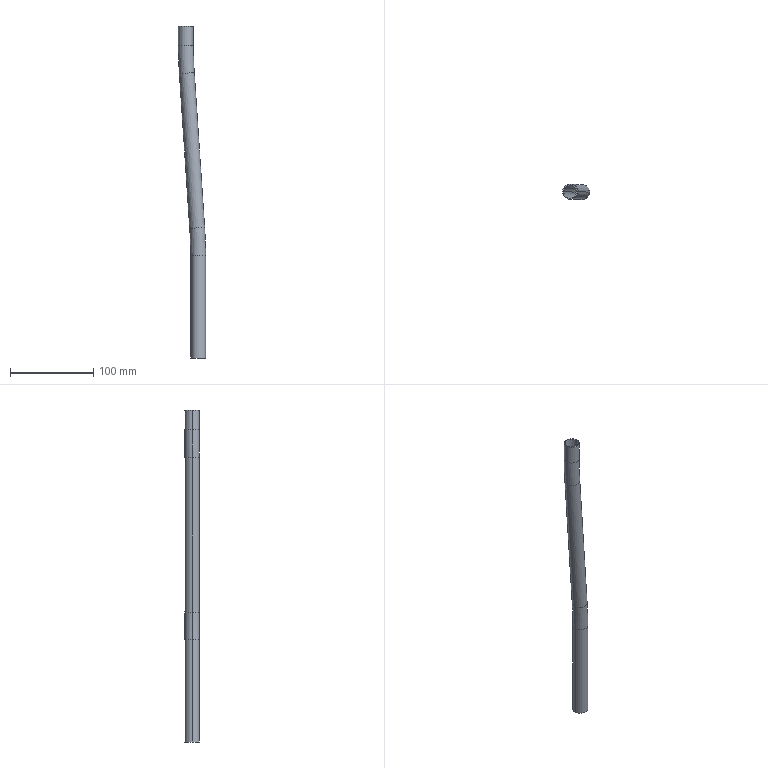Part | STEP file | Upper Chain Tube | 1 solid | 22 faces | box 32.75 x 18 x 400 mm | volume 21388 mm3 | cylinder 12 | torus 8 | plane 2 | commonest cylinder face diameters 16 x6 18 x6
STEP:
#1=CARTESIAN_POINT('',(0.,0.,0.));
#2=DIRECTION('',(0.,0.,1.));
#3=DIRECTION('',(1.,0.,0.));
#4=AXIS2_PLACEMENT_3D('',#1,#2,#3);
#5=CARTESIAN_POINT('',(-8.,0.,23.257));
#6=VERTEX_POINT('',#5);
#7=CARTESIAN_POINT('',(-9.102,0.,56.17));
#8=VERTEX_POINT('',#7);
#9=CARTESIAN_POINT('',(-500.,0.,23.257));
#10=DIRECTION('',(0.,-1.,0.));
#11=DIRECTION('',(0.,0.,-1.));
#12=AXIS2_PLACEMENT_3D('',#9,#10,#11);
#13=CIRCLE('',#12,492.);
#14=CARTESIAN_POINT('',(-500.,0.,23.257));
#15=DIRECTION('',(0.,-1.,0.));
#16=DIRECTION('',(0.,0.,-1.));
#17=AXIS2_PLACEMENT_3D('',#14,#15,#16);
#18=TOROIDAL_SURFACE('',#17,500.,8.);
#19=CARTESIAN_POINT('',(0.,3.142));
#20=DIRECTION('',(1.,0.));
#21=VECTOR('',#20,1.);
#22=LINE('',#19,#21);
#23=(GEOMETRIC_REPRESENTATION_CONTEXT(2)PARAMETRIC_REPRESENTATION_CONTEXT()REPRESENTATION_CONTEXT('',''));
#24=DEFINITIONAL_REPRESENTATION('',(#22),#23);
#25=PCURVE('',#18,#24);
#26=CARTESIAN_POINT('',(-500.,0.,23.257));
#27=DIRECTION('',(0.,-1.,0.));
#28=DIRECTION('',(0.,0.,-1.));
#29=AXIS2_PLACEMENT_3D('',#26,#27,#28);
#30=TOROIDAL_SURFACE('',#29,500.,8.);
#31=CARTESIAN_POINT('',(0.,3.142));
#32=DIRECTION('',(1.,0.));
#33=VECTOR('',#32,1.);
#34=LINE('',#31,#33);
#35=(GEOMETRIC_REPRESENTATION_CONTEXT(2)PARAMETRIC_REPRESENTATION_CONTEXT()REPRESENTATION_CONTEXT('',''));
#36=DEFINITIONAL_REPRESENTATION('',(#34),#35);
#37=PCURVE('',#30,#36);
#38=SURFACE_CURVE('',#13,(#25,#37),.PCURVE_S1.);
#39=EDGE_CURVE('',#6,#8,#38,.T.);
#40=ORIENTED_EDGE('',*,*,#39,.T.);
#41=CARTESIAN_POINT('',(6.862,0.,57.24));
#42=VERTEX_POINT('',#41);
#43=CARTESIAN_POINT('',(-1.12,0.,56.705));
#44=DIRECTION('',(-0.0669,0.,0.9978));
#45=DIRECTION('',(0.9978,0.,0.0669));
#46=AXIS2_PLACEMENT_3D('',#43,#44,#45);
#47=CIRCLE('',#46,8.);
#48=CARTESIAN_POINT('',(1.638,6.283));
#49=DIRECTION('',(0.,-1.));
#50=VECTOR('',#49,1.);
#51=LINE('',#48,#50);
#52=(GEOMETRIC_REPRESENTATION_CONTEXT(2)PARAMETRIC_REPRESENTATION_CONTEXT()REPRESENTATION_CONTEXT('',''));
#53=DEFINITIONAL_REPRESENTATION('',(#51),#52);
#54=PCURVE('',#18,#53);
#55=CARTESIAN_POINT('',(-1.12,0.,56.705));
#56=DIRECTION('',(-0.0669,0.,0.9978));
#57=DIRECTION('',(0.9978,0.,0.0669));
#58=AXIS2_PLACEMENT_3D('',#55,#56,#57);
#59=CYLINDRICAL_SURFACE('',#58,8.);
#60=CARTESIAN_POINT('',(0.,0.));
#61=DIRECTION('',(1.,0.));
#62=VECTOR('',#61,1.);
#63=LINE('',#60,#62);
#64=(GEOMETRIC_REPRESENTATION_CONTEXT(2)PARAMETRIC_REPRESENTATION_CONTEXT()REPRESENTATION_CONTEXT('',''));
#65=DEFINITIONAL_REPRESENTATION('',(#63),#64);
#66=PCURVE('',#59,#65);
#67=SURFACE_CURVE('',#47,(#54,#66),.PCURVE_S1.);
#68=EDGE_CURVE('',#42,#8,#67,.T.);
#69=ORIENTED_EDGE('',*,*,#68,.F.);
#70=CARTESIAN_POINT('',(8.,0.,23.257));
#71=VERTEX_POINT('',#70);
#72=CARTESIAN_POINT('',(-500.,0.,23.257));
#73=DIRECTION('',(0.,-1.,0.));
#74=DIRECTION('',(0.,0.,-1.));
#75=AXIS2_PLACEMENT_3D('',#72,#73,#74);
#76=CIRCLE('',#75,508.);
#77=CARTESIAN_POINT('',(0.,6.283));
#78=DIRECTION('',(1.,0.));
#79=VECTOR('',#78,1.);
#80=LINE('',#77,#79);
#81=(GEOMETRIC_REPRESENTATION_CONTEXT(2)PARAMETRIC_REPRESENTATION_CONTEXT()REPRESENTATION_CONTEXT('',''));
#82=DEFINITIONAL_REPRESENTATION('',(#80),#81);
#83=PCURVE('',#18,#82);
#84=CARTESIAN_POINT('',(0.,0.));
#85=DIRECTION('',(1.,0.));
#86=VECTOR('',#85,1.);
#87=LINE('',#84,#86);
#88=(GEOMETRIC_REPRESENTATION_CONTEXT(2)PARAMETRIC_REPRESENTATION_CONTEXT()REPRESENTATION_CONTEXT('',''));
#89=DEFINITIONAL_REPRESENTATION('',(#87),#88);
#90=PCURVE('',#30,#89);
#91=SURFACE_CURVE('',#76,(#83,#90),.PCURVE_S1.);
#92=EDGE_CURVE('',#71,#42,#91,.T.);
#93=ORIENTED_EDGE('',*,*,#92,.F.);
#94=CARTESIAN_POINT('',(0.,0.,23.257));
#95=DIRECTION('',(0.,0.,1.));
#96=DIRECTION('',(1.,0.,0.));
#97=AXIS2_PLACEMENT_3D('',#94,#95,#96);
#98=CIRCLE('',#97,8.);
#99=CARTESIAN_POINT('',(1.571,6.283));
#100=DIRECTION('',(0.,-1.));
#101=VECTOR('',#100,1.);
#102=LINE('',#99,#101);
#103=(GEOMETRIC_REPRESENTATION_CONTEXT(2)PARAMETRIC_REPRESENTATION_CONTEXT()REPRESENTATION_CONTEXT('',''));
#104=DEFINITIONAL_REPRESENTATION('',(#102),#103);
#105=PCURVE('',#18,#104);
#106=CARTESIAN_POINT('',(0.,0.,-100.));
#107=DIRECTION('',(0.,0.,1.));
#108=DIRECTION('',(1.,0.,0.));
#109=AXIS2_PLACEMENT_3D('',#106,#107,#108);
#110=CYLINDRICAL_SURFACE('',#109,8.);
#111=CARTESIAN_POINT('',(0.,123.257));
#112=DIRECTION('',(1.,0.));
#113=VECTOR('',#112,1.);
#114=LINE('',#111,#113);
#115=(GEOMETRIC_REPRESENTATION_CONTEXT(2)PARAMETRIC_REPRESENTATION_CONTEXT()REPRESENTATION_CONTEXT('',''));
#116=DEFINITIONAL_REPRESENTATION('',(#114),#115);
#117=PCURVE('',#110,#116);
#118=SURFACE_CURVE('',#98,(#105,#117),.PCURVE_S1.);
#119=EDGE_CURVE('',#71,#6,#118,.T.);
#120=ORIENTED_EDGE('',*,*,#119,.T.);
#121=EDGE_LOOP('',(#40,#69,#93,#120));
#122=FACE_BOUND('',#121,.F.);
#123=ADVANCED_FACE('',(#122),#18,.F.);
#124=CARTESIAN_POINT('',(-9.,0.,23.257));
#125=VERTEX_POINT('',#124);
#126=CARTESIAN_POINT('',(9.,0.,23.257));
#127=VERTEX_POINT('',#126);
#128=CARTESIAN_POINT('',(0.,0.,23.257));
#129=DIRECTION('',(0.,0.,1.));
#130=DIRECTION('',(1.,0.,0.));
#131=AXIS2_PLACEMENT_3D('',#128,#129,#130);
#132=CIRCLE('',#131,9.);
#133=CARTESIAN_POINT('',(-500.,0.,23.257));
#134=DIRECTION('',(0.,-1.,0.));
#135=DIRECTION('',(0.,0.,-1.));
#136=AXIS2_PLACEMENT_3D('',#133,#134,#135);
#137=TOROIDAL_SURFACE('',#136,500.,9.);
#138=CARTESIAN_POINT('',(1.571,6.283));
#139=DIRECTION('',(0.,-1.));
#140=VECTOR('',#139,1.);
#141=LINE('',#138,#140);
#142=(GEOMETRIC_REPRESENTATION_CONTEXT(2)PARAMETRIC_REPRESENTATION_CONTEXT()REPRESENTATION_CONTEXT('',''));
#143=DEFINITIONAL_REPRESENTATION('',(#141),#142);
#144=PCURVE('',#137,#143);
#145=CARTESIAN_POINT('',(0.,0.,-100.));
#146=DIRECTION('',(0.,0.,1.));
#147=DIRECTION('',(1.,0.,0.));
#148=AXIS2_PLACEMENT_3D('',#145,#146,#147);
#149=CYLINDRICAL_SURFACE('',#148,9.);
#150=CARTESIAN_POINT('',(0.,123.257));
#151=DIRECTION('',(1.,0.));
#152=VECTOR('',#151,1.);
#153=LINE('',#150,#152);
#154=(GEOMETRIC_REPRESENTATION_CONTEXT(2)PARAMETRIC_REPRESENTATION_CONTEXT()REPRESENTATION_CONTEXT('',''));
#155=DEFINITIONAL_REPRESENTATION('',(#153),#154);
#156=PCURVE('',#149,#155);
#157=SURFACE_CURVE('',#132,(#144,#156),.PCURVE_S1.);
#158=EDGE_CURVE('',#125,#127,#157,.T.);
#159=ORIENTED_EDGE('',*,*,#158,.T.);
#160=CARTESIAN_POINT('',(7.86,0.,57.307));
#161=VERTEX_POINT('',#160);
#162=CARTESIAN_POINT('',(-500.,0.,23.257));
#163=DIRECTION('',(0.,-1.,0.));
#164=DIRECTION('',(0.,0.,-1.));
#165=AXIS2_PLACEMENT_3D('',#162,#163,#164);
#166=CIRCLE('',#165,509.);
#167=CARTESIAN_POINT('',(0.,0.));
#168=DIRECTION('',(1.,0.));
#169=VECTOR('',#168,1.);
#170=LINE('',#167,#169);
#171=(GEOMETRIC_REPRESENTATION_CONTEXT(2)PARAMETRIC_REPRESENTATION_CONTEXT()REPRESENTATION_CONTEXT('',''));
#172=DEFINITIONAL_REPRESENTATION('',(#170),#171);
#173=PCURVE('',#137,#172);
#174=CARTESIAN_POINT('',(-500.,0.,23.257));
#175=DIRECTION('',(0.,-1.,0.));
#176=DIRECTION('',(0.,0.,-1.));
#177=AXIS2_PLACEMENT_3D('',#174,#175,#176);
#178=TOROIDAL_SURFACE('',#177,500.,9.);
#179=CARTESIAN_POINT('',(0.,6.283));
#180=DIRECTION('',(1.,0.));
#181=VECTOR('',#180,1.);
#182=LINE('',#179,#181);
#183=(GEOMETRIC_REPRESENTATION_CONTEXT(2)PARAMETRIC_REPRESENTATION_CONTEXT()REPRESENTATION_CONTEXT('',''));
#184=DEFINITIONAL_REPRESENTATION('',(#182),#183);
#185=PCURVE('',#178,#184);
#186=SURFACE_CURVE('',#166,(#173,#185),.PCURVE_S1.);
#187=EDGE_CURVE('',#127,#161,#186,.T.);
#188=ORIENTED_EDGE('',*,*,#187,.T.);
#189=CARTESIAN_POINT('',(-10.1,0.,56.103));
#190=VERTEX_POINT('',#189);
#191=CARTESIAN_POINT('',(-1.12,0.,56.705));
#192=DIRECTION('',(-0.0669,0.,0.9978));
#193=DIRECTION('',(0.9978,0.,0.0669));
#194=AXIS2_PLACEMENT_3D('',#191,#192,#193);
#195=CIRCLE('',#194,9.);
#196=CARTESIAN_POINT('',(1.638,6.283));
#197=DIRECTION('',(0.,-1.));
#198=VECTOR('',#197,1.);
#199=LINE('',#196,#198);
#200=(GEOMETRIC_REPRESENTATION_CONTEXT(2)PARAMETRIC_REPRESENTATION_CONTEXT()REPRESENTATION_CONTEXT('',''));
#201=DEFINITIONAL_REPRESENTATION('',(#199),#200);
#202=PCURVE('',#137,#201);
#203=CARTESIAN_POINT('',(-1.12,0.,56.705));
#204=DIRECTION('',(-0.0669,0.,0.9978));
#205=DIRECTION('',(0.9978,0.,0.0669));
#206=AXIS2_PLACEMENT_3D('',#203,#204,#205);
#207=CYLINDRICAL_SURFACE('',#206,9.);
#208=CARTESIAN_POINT('',(0.,0.));
#209=DIRECTION('',(1.,0.));
#210=VECTOR('',#209,1.);
#211=LINE('',#208,#210);
#212=(GEOMETRIC_REPRESENTATION_CONTEXT(2)PARAMETRIC_REPRESENTATION_CONTEXT()REPRESENTATION_CONTEXT('',''));
#213=DEFINITIONAL_REPRESENTATION('',(#211),#212);
#214=PCURVE('',#207,#213);
#215=SURFACE_CURVE('',#195,(#202,#214),.PCURVE_S1.);
#216=EDGE_CURVE('',#190,#161,#215,.T.);
#217=ORIENTED_EDGE('',*,*,#216,.F.);
#218=CARTESIAN_POINT('',(-500.,0.,23.257));
#219=DIRECTION('',(0.,-1.,0.));
#220=DIRECTION('',(0.,0.,-1.));
#221=AXIS2_PLACEMENT_3D('',#218,#219,#220);
#222=CIRCLE('',#221,491.);
#223=CARTESIAN_POINT('',(0.,3.142));
#224=DIRECTION('',(1.,0.));
#225=VECTOR('',#224,1.);
#226=LINE('',#223,#225);
#227=(GEOMETRIC_REPRESENTATION_CONTEXT(2)PARAMETRIC_REPRESENTATION_CONTEXT()REPRESENTATION_CONTEXT('',''));
#228=DEFINITIONAL_REPRESENTATION('',(#226),#227);
#229=PCURVE('',#137,#228);
#230=CARTESIAN_POINT('',(0.,3.142));
#231=DIRECTION('',(1.,0.));
#232=VECTOR('',#231,1.);
#233=LINE('',#230,#232);
#234=(GEOMETRIC_REPRESENTATION_CONTEXT(2)PARAMETRIC_REPRESENTATION_CONTEXT()REPRESENTATION_CONTEXT('',''));
#235=DEFINITIONAL_REPRESENTATION('',(#233),#234);
#236=PCURVE('',#178,#235);
#237=SURFACE_CURVE('',#222,(#229,#236),.PCURVE_S1.);
#238=EDGE_CURVE('',#125,#190,#237,.T.);
#239=ORIENTED_EDGE('',*,*,#238,.F.);
#240=EDGE_LOOP('',(#159,#188,#217,#239));
#241=FACE_BOUND('',#240,.T.);
#242=ADVANCED_FACE('',(#241),#137,.T.);
#243=CARTESIAN_POINT('',(-5.648,0.,243.83));
#244=VERTEX_POINT('',#243);
#245=CARTESIAN_POINT('',(-6.75,0.,276.743));
#246=VERTEX_POINT('',#245);
#247=CARTESIAN_POINT('',(485.25,0.,276.743));
#248=DIRECTION('',(0.,1.,0.));
#249=DIRECTION('',(0.,0.,1.));
#250=AXIS2_PLACEMENT_3D('',#247,#248,#249);
#251=CIRCLE('',#250,492.);
#252=CARTESIAN_POINT('',(485.25,0.,276.743));
#253=DIRECTION('',(0.,1.,0.));
#254=DIRECTION('',(0.,0.,1.));
#255=AXIS2_PLACEMENT_3D('',#252,#253,#254);
#256=TOROIDAL_SURFACE('',#255,500.,8.);
#257=CARTESIAN_POINT('',(0.,3.142));
#258=DIRECTION('',(1.,0.));
#259=VECTOR('',#258,1.);
#260=LINE('',#257,#259);
#261=(GEOMETRIC_REPRESENTATION_CONTEXT(2)PARAMETRIC_REPRESENTATION_CONTEXT()REPRESENTATION_CONTEXT('',''));
#262=DEFINITIONAL_REPRESENTATION('',(#260),#261);
#263=PCURVE('',#256,#262);
#264=CARTESIAN_POINT('',(485.25,0.,276.743));
#265=DIRECTION('',(0.,1.,0.));
#266=DIRECTION('',(0.,0.,1.));
#267=AXIS2_PLACEMENT_3D('',#264,#265,#266);
#268=TOROIDAL_SURFACE('',#267,500.,8.);
#269=CARTESIAN_POINT('',(0.,3.142));
#270=DIRECTION('',(1.,0.));
#271=VECTOR('',#270,1.);
#272=LINE('',#269,#271);
#273=(GEOMETRIC_REPRESENTATION_CONTEXT(2)PARAMETRIC_REPRESENTATION_CONTEXT()REPRESENTATION_CONTEXT('',''));
#274=DEFINITIONAL_REPRESENTATION('',(#272),#273);
#275=PCURVE('',#268,#274);
#276=SURFACE_CURVE('',#251,(#263,#275),.PCURVE_S1.);
#277=EDGE_CURVE('',#244,#246,#276,.T.);
#278=ORIENTED_EDGE('',*,*,#277,.T.);
#279=CARTESIAN_POINT('',(-22.75,0.,276.743));
#280=VERTEX_POINT('',#279);
#281=CARTESIAN_POINT('',(-14.75,0.,276.743));
#282=DIRECTION('',(0.,0.,1.));
#283=DIRECTION('',(1.,0.,0.));
#284=AXIS2_PLACEMENT_3D('',#281,#282,#283);
#285=CIRCLE('',#284,8.);
#286=CARTESIAN_POINT('',(4.712,9.425));
#287=DIRECTION('',(0.,-1.));
#288=VECTOR('',#287,1.);
#289=LINE('',#286,#288);
#290=(GEOMETRIC_REPRESENTATION_CONTEXT(2)PARAMETRIC_REPRESENTATION_CONTEXT()REPRESENTATION_CONTEXT('',''));
#291=DEFINITIONAL_REPRESENTATION('',(#289),#290);
#292=PCURVE('',#256,#291);
#293=CARTESIAN_POINT('',(-14.75,0.,276.743));
#294=DIRECTION('',(0.,0.,1.));
#295=DIRECTION('',(1.,0.,0.));
#296=AXIS2_PLACEMENT_3D('',#293,#294,#295);
#297=CYLINDRICAL_SURFACE('',#296,8.);
#298=CARTESIAN_POINT('',(0.,0.));
#299=DIRECTION('',(1.,0.));
#300=VECTOR('',#299,1.);
#301=LINE('',#298,#300);
#302=(GEOMETRIC_REPRESENTATION_CONTEXT(2)PARAMETRIC_REPRESENTATION_CONTEXT()REPRESENTATION_CONTEXT('',''));
#303=DEFINITIONAL_REPRESENTATION('',(#301),#302);
#304=PCURVE('',#297,#303);
#305=SURFACE_CURVE('',#285,(#292,#304),.PCURVE_S1.);
#306=EDGE_CURVE('',#280,#246,#305,.T.);
#307=ORIENTED_EDGE('',*,*,#306,.F.);
#308=CARTESIAN_POINT('',(-21.612,0.,242.76));
#309=VERTEX_POINT('',#308);
#310=CARTESIAN_POINT('',(485.25,0.,276.743));
#311=DIRECTION('',(0.,1.,0.));
#312=DIRECTION('',(0.,0.,1.));
#313=AXIS2_PLACEMENT_3D('',#310,#311,#312);
#314=CIRCLE('',#313,508.);
#315=CARTESIAN_POINT('',(0.,6.283));
#316=DIRECTION('',(1.,0.));
#317=VECTOR('',#316,1.);
#318=LINE('',#315,#317);
#319=(GEOMETRIC_REPRESENTATION_CONTEXT(2)PARAMETRIC_REPRESENTATION_CONTEXT()REPRESENTATION_CONTEXT('',''));
#320=DEFINITIONAL_REPRESENTATION('',(#318),#319);
#321=PCURVE('',#256,#320);
#322=CARTESIAN_POINT('',(0.,0.));
#323=DIRECTION('',(1.,0.));
#324=VECTOR('',#323,1.);
#325=LINE('',#322,#324);
#326=(GEOMETRIC_REPRESENTATION_CONTEXT(2)PARAMETRIC_REPRESENTATION_CONTEXT()REPRESENTATION_CONTEXT('',''));
#327=DEFINITIONAL_REPRESENTATION('',(#325),#326);
#328=PCURVE('',#268,#327);
#329=SURFACE_CURVE('',#314,(#321,#328),.PCURVE_S1.);
#330=EDGE_CURVE('',#309,#280,#329,.T.);
#331=ORIENTED_EDGE('',*,*,#330,.F.);
#332=CARTESIAN_POINT('',(-13.63,0.,243.295));
#333=DIRECTION('',(-0.0669,0.,0.9978));
#334=DIRECTION('',(0.9978,0.,0.0669));
#335=AXIS2_PLACEMENT_3D('',#332,#333,#334);
#336=CIRCLE('',#335,8.);
#337=CARTESIAN_POINT('',(4.645,9.425));
#338=DIRECTION('',(0.,-1.));
#339=VECTOR('',#338,1.);
#340=LINE('',#337,#339);
#341=(GEOMETRIC_REPRESENTATION_CONTEXT(2)PARAMETRIC_REPRESENTATION_CONTEXT()REPRESENTATION_CONTEXT('',''));
#342=DEFINITIONAL_REPRESENTATION('',(#340),#341);
#343=PCURVE('',#256,#342);
#344=CARTESIAN_POINT('',(-1.12,0.,56.705));
#345=DIRECTION('',(-0.0669,0.,0.9978));
#346=DIRECTION('',(0.9978,0.,0.0669));
#347=AXIS2_PLACEMENT_3D('',#344,#345,#346);
#348=CYLINDRICAL_SURFACE('',#347,8.);
#349=CARTESIAN_POINT('',(0.,187.009));
#350=DIRECTION('',(1.,0.));
#351=VECTOR('',#350,1.);
#352=LINE('',#349,#351);
#353=(GEOMETRIC_REPRESENTATION_CONTEXT(2)PARAMETRIC_REPRESENTATION_CONTEXT()REPRESENTATION_CONTEXT('',''));
#354=DEFINITIONAL_REPRESENTATION('',(#352),#353);
#355=PCURVE('',#348,#354);
#356=SURFACE_CURVE('',#336,(#343,#355),.PCURVE_S1.);
#357=EDGE_CURVE('',#309,#244,#356,.T.);
#358=ORIENTED_EDGE('',*,*,#357,.T.);
#359=EDGE_LOOP('',(#278,#307,#331,#358));
#360=FACE_BOUND('',#359,.F.);
#361=ADVANCED_FACE('',(#360),#256,.F.);
#362=CARTESIAN_POINT('',(-4.65,0.,243.897));
#363=VERTEX_POINT('',#362);
#364=CARTESIAN_POINT('',(-22.61,0.,242.693));
#365=VERTEX_POINT('',#364);
#366=CARTESIAN_POINT('',(-13.63,0.,243.295));
#367=DIRECTION('',(-0.0669,0.,0.9978));
#368=DIRECTION('',(0.9978,0.,0.0669));
#369=AXIS2_PLACEMENT_3D('',#366,#367,#368);
#370=CIRCLE('',#369,9.);
#371=CARTESIAN_POINT('',(485.25,0.,276.743));
#372=DIRECTION('',(0.,1.,0.));
#373=DIRECTION('',(0.,0.,1.));
#374=AXIS2_PLACEMENT_3D('',#371,#372,#373);
#375=TOROIDAL_SURFACE('',#374,500.,9.);
#376=CARTESIAN_POINT('',(4.645,3.142));
#377=DIRECTION('',(0.,-1.));
#378=VECTOR('',#377,1.);
#379=LINE('',#376,#378);
#380=(GEOMETRIC_REPRESENTATION_CONTEXT(2)PARAMETRIC_REPRESENTATION_CONTEXT()REPRESENTATION_CONTEXT('',''));
#381=DEFINITIONAL_REPRESENTATION('',(#379),#380);
#382=PCURVE('',#375,#381);
#383=CARTESIAN_POINT('',(-1.12,0.,56.705));
#384=DIRECTION('',(-0.0669,0.,0.9978));
#385=DIRECTION('',(0.9978,0.,0.0669));
#386=AXIS2_PLACEMENT_3D('',#383,#384,#385);
#387=CYLINDRICAL_SURFACE('',#386,9.);
#388=CARTESIAN_POINT('',(0.,187.009));
#389=DIRECTION('',(1.,0.));
#390=VECTOR('',#389,1.);
#391=LINE('',#388,#390);
#392=(GEOMETRIC_REPRESENTATION_CONTEXT(2)PARAMETRIC_REPRESENTATION_CONTEXT()REPRESENTATION_CONTEXT('',''));
#393=DEFINITIONAL_REPRESENTATION('',(#391),#392);
#394=PCURVE('',#387,#393);
#395=SURFACE_CURVE('',#370,(#382,#394),.PCURVE_S1.);
#396=EDGE_CURVE('',#363,#365,#395,.T.);
#397=ORIENTED_EDGE('',*,*,#396,.T.);
#398=CARTESIAN_POINT('',(-23.75,0.,276.743));
#399=VERTEX_POINT('',#398);
#400=CARTESIAN_POINT('',(485.25,0.,276.743));
#401=DIRECTION('',(0.,1.,0.));
#402=DIRECTION('',(0.,0.,1.));
#403=AXIS2_PLACEMENT_3D('',#400,#401,#402);
#404=CIRCLE('',#403,509.);
#405=CARTESIAN_POINT('',(0.,0.));
#406=DIRECTION('',(1.,0.));
#407=VECTOR('',#406,1.);
#408=LINE('',#405,#407);
#409=(GEOMETRIC_REPRESENTATION_CONTEXT(2)PARAMETRIC_REPRESENTATION_CONTEXT()REPRESENTATION_CONTEXT('',''));
#410=DEFINITIONAL_REPRESENTATION('',(#408),#409);
#411=PCURVE('',#375,#410);
#412=CARTESIAN_POINT('',(485.25,0.,276.743));
#413=DIRECTION('',(0.,1.,0.));
#414=DIRECTION('',(0.,0.,1.));
#415=AXIS2_PLACEMENT_3D('',#412,#413,#414);
#416=TOROIDAL_SURFACE('',#415,500.,9.);
#417=CARTESIAN_POINT('',(0.,6.283));
#418=DIRECTION('',(1.,0.));
#419=VECTOR('',#418,1.);
#420=LINE('',#417,#419);
#421=(GEOMETRIC_REPRESENTATION_CONTEXT(2)PARAMETRIC_REPRESENTATION_CONTEXT()REPRESENTATION_CONTEXT('',''));
#422=DEFINITIONAL_REPRESENTATION('',(#420),#421);
#423=PCURVE('',#416,#422);
#424=SURFACE_CURVE('',#404,(#411,#423),.PCURVE_S1.);
#425=EDGE_CURVE('',#365,#399,#424,.T.);
#426=ORIENTED_EDGE('',*,*,#425,.T.);
#427=CARTESIAN_POINT('',(-5.75,0.,276.743));
#428=VERTEX_POINT('',#427);
#429=CARTESIAN_POINT('',(-14.75,0.,276.743));
#430=DIRECTION('',(0.,0.,1.));
#431=DIRECTION('',(1.,0.,0.));
#432=AXIS2_PLACEMENT_3D('',#429,#430,#431);
#433=CIRCLE('',#432,9.);
#434=CARTESIAN_POINT('',(4.712,3.142));
#435=DIRECTION('',(0.,-1.));
#436=VECTOR('',#435,1.);
#437=LINE('',#434,#436);
#438=(GEOMETRIC_REPRESENTATION_CONTEXT(2)PARAMETRIC_REPRESENTATION_CONTEXT()REPRESENTATION_CONTEXT('',''));
#439=DEFINITIONAL_REPRESENTATION('',(#437),#438);
#440=PCURVE('',#375,#439);
#441=CARTESIAN_POINT('',(-14.75,0.,276.743));
#442=DIRECTION('',(0.,0.,1.));
#443=DIRECTION('',(1.,0.,0.));
#444=AXIS2_PLACEMENT_3D('',#441,#442,#443);
#445=CYLINDRICAL_SURFACE('',#444,9.);
#446=CARTESIAN_POINT('',(0.,0.));
#447=DIRECTION('',(1.,0.));
#448=VECTOR('',#447,1.);
#449=LINE('',#446,#448);
#450=(GEOMETRIC_REPRESENTATION_CONTEXT(2)PARAMETRIC_REPRESENTATION_CONTEXT()REPRESENTATION_CONTEXT('',''));
#451=DEFINITIONAL_REPRESENTATION('',(#449),#450);
#452=PCURVE('',#445,#451);
#453=SURFACE_CURVE('',#433,(#440,#452),.PCURVE_S1.);
#454=EDGE_CURVE('',#428,#399,#453,.T.);
#455=ORIENTED_EDGE('',*,*,#454,.F.);
#456=CARTESIAN_POINT('',(485.25,0.,276.743));
#457=DIRECTION('',(0.,1.,0.));
#458=DIRECTION('',(0.,0.,1.));
#459=AXIS2_PLACEMENT_3D('',#456,#457,#458);
#460=CIRCLE('',#459,491.);
#461=CARTESIAN_POINT('',(0.,3.142));
#462=DIRECTION('',(1.,0.));
#463=VECTOR('',#462,1.);
#464=LINE('',#461,#463);
#465=(GEOMETRIC_REPRESENTATION_CONTEXT(2)PARAMETRIC_REPRESENTATION_CONTEXT()REPRESENTATION_CONTEXT('',''));
#466=DEFINITIONAL_REPRESENTATION('',(#464),#465);
#467=PCURVE('',#375,#466);
#468=CARTESIAN_POINT('',(0.,3.142));
#469=DIRECTION('',(1.,0.));
#470=VECTOR('',#469,1.);
#471=LINE('',#468,#470);
#472=(GEOMETRIC_REPRESENTATION_CONTEXT(2)PARAMETRIC_REPRESENTATION_CONTEXT()REPRESENTATION_CONTEXT('',''));
#473=DEFINITIONAL_REPRESENTATION('',(#471),#472);
#474=PCURVE('',#416,#473);
#475=SURFACE_CURVE('',#460,(#467,#474),.PCURVE_S1.);
#476=EDGE_CURVE('',#363,#428,#475,.T.);
#477=ORIENTED_EDGE('',*,*,#476,.F.);
#478=EDGE_LOOP('',(#397,#426,#455,#477));
#479=FACE_BOUND('',#478,.T.);
#480=ADVANCED_FACE('',(#479),#375,.T.);
#481=CARTESIAN_POINT('',(6.862,0.,57.24));
#482=DIRECTION('',(-0.0669,0.,0.9978));
#483=VECTOR('',#482,1.);
#484=LINE('',#481,#483);
#485=CARTESIAN_POINT('',(6.283,0.));
#486=DIRECTION('',(0.,1.));
#487=VECTOR('',#486,1.);
#488=LINE('',#485,#487);
#489=(GEOMETRIC_REPRESENTATION_CONTEXT(2)PARAMETRIC_REPRESENTATION_CONTEXT()REPRESENTATION_CONTEXT('',''));
#490=DEFINITIONAL_REPRESENTATION('',(#488),#489);
#491=PCURVE('',#348,#490);
#492=CARTESIAN_POINT('',(0.,0.));
#493=DIRECTION('',(0.,1.));
#494=VECTOR('',#493,1.);
#495=LINE('',#492,#494);
#496=(GEOMETRIC_REPRESENTATION_CONTEXT(2)PARAMETRIC_REPRESENTATION_CONTEXT()REPRESENTATION_CONTEXT('',''));
#497=DEFINITIONAL_REPRESENTATION('',(#495),#496);
#498=PCURVE('',#59,#497);
#499=SURFACE_CURVE('',#484,(#491,#498),.PCURVE_S1.);
#500=EDGE_CURVE('',#42,#244,#499,.T.);
#501=ORIENTED_EDGE('',*,*,#500,.T.);
#502=ORIENTED_EDGE('',*,*,#357,.F.);
#503=CARTESIAN_POINT('',(-9.102,0.,56.17));
#504=DIRECTION('',(-0.0669,0.,0.9978));
#505=VECTOR('',#504,1.);
#506=LINE('',#503,#505);
#507=CARTESIAN_POINT('',(3.142,0.));
#508=DIRECTION('',(0.,1.));
#509=VECTOR('',#508,1.);
#510=LINE('',#507,#509);
#511=(GEOMETRIC_REPRESENTATION_CONTEXT(2)PARAMETRIC_REPRESENTATION_CONTEXT()REPRESENTATION_CONTEXT('',''));
#512=DEFINITIONAL_REPRESENTATION('',(#510),#511);
#513=PCURVE('',#348,#512);
#514=CARTESIAN_POINT('',(3.142,0.));
#515=DIRECTION('',(0.,1.));
#516=VECTOR('',#515,1.);
#517=LINE('',#514,#516);
#518=(GEOMETRIC_REPRESENTATION_CONTEXT(2)PARAMETRIC_REPRESENTATION_CONTEXT()REPRESENTATION_CONTEXT('',''));
#519=DEFINITIONAL_REPRESENTATION('',(#517),#518);
#520=PCURVE('',#59,#519);
#521=SURFACE_CURVE('',#506,(#513,#520),.PCURVE_S1.);
#522=EDGE_CURVE('',#8,#309,#521,.T.);
#523=ORIENTED_EDGE('',*,*,#522,.F.);
#524=CARTESIAN_POINT('',(-1.12,0.,56.705));
#525=DIRECTION('',(-0.0669,0.,0.9978));
#526=DIRECTION('',(0.9978,0.,0.0669));
#527=AXIS2_PLACEMENT_3D('',#524,#525,#526);
#528=CIRCLE('',#527,8.);
#529=CARTESIAN_POINT('',(0.,0.));
#530=DIRECTION('',(1.,0.));
#531=VECTOR('',#530,1.);
#532=LINE('',#529,#531);
#533=(GEOMETRIC_REPRESENTATION_CONTEXT(2)PARAMETRIC_REPRESENTATION_CONTEXT()REPRESENTATION_CONTEXT('',''));
#534=DEFINITIONAL_REPRESENTATION('',(#532),#533);
#535=PCURVE('',#348,#534);
#536=CARTESIAN_POINT('',(1.638,6.283));
#537=DIRECTION('',(0.,-1.));
#538=VECTOR('',#537,1.);
#539=LINE('',#536,#538);
#540=(GEOMETRIC_REPRESENTATION_CONTEXT(2)PARAMETRIC_REPRESENTATION_CONTEXT()REPRESENTATION_CONTEXT('',''));
#541=DEFINITIONAL_REPRESENTATION('',(#539),#540);
#542=PCURVE('',#30,#541);
#543=SURFACE_CURVE('',#528,(#535,#542),.PCURVE_S1.);
#544=EDGE_CURVE('',#8,#42,#543,.T.);
#545=ORIENTED_EDGE('',*,*,#544,.T.);
#546=EDGE_LOOP('',(#501,#502,#523,#545));
#547=FACE_BOUND('',#546,.F.);
#548=ADVANCED_FACE('',(#547),#348,.F.);
#549=CARTESIAN_POINT('',(-1.12,0.,56.705));
#550=DIRECTION('',(-0.0669,0.,0.9978));
#551=DIRECTION('',(0.9978,0.,0.0669));
#552=AXIS2_PLACEMENT_3D('',#549,#550,#551);
#553=CIRCLE('',#552,9.);
#554=CARTESIAN_POINT('',(0.,0.));
#555=DIRECTION('',(1.,0.));
#556=VECTOR('',#555,1.);
#557=LINE('',#554,#556);
#558=(GEOMETRIC_REPRESENTATION_CONTEXT(2)PARAMETRIC_REPRESENTATION_CONTEXT()REPRESENTATION_CONTEXT('',''));
#559=DEFINITIONAL_REPRESENTATION('',(#557),#558);
#560=PCURVE('',#387,#559);
#561=CARTESIAN_POINT('',(1.638,6.283));
#562=DIRECTION('',(0.,-1.));
#563=VECTOR('',#562,1.);
#564=LINE('',#561,#563);
#565=(GEOMETRIC_REPRESENTATION_CONTEXT(2)PARAMETRIC_REPRESENTATION_CONTEXT()REPRESENTATION_CONTEXT('',''));
#566=DEFINITIONAL_REPRESENTATION('',(#564),#565);
#567=PCURVE('',#178,#566);
#568=SURFACE_CURVE('',#553,(#560,#567),.PCURVE_S1.);
#569=EDGE_CURVE('',#161,#190,#568,.T.);
#570=ORIENTED_EDGE('',*,*,#569,.T.);
#571=CARTESIAN_POINT('',(-10.1,0.,56.103));
#572=DIRECTION('',(-0.0669,0.,0.9978));
#573=VECTOR('',#572,1.);
#574=LINE('',#571,#573);
#575=CARTESIAN_POINT('',(3.142,0.));
#576=DIRECTION('',(0.,1.));
#577=VECTOR('',#576,1.);
#578=LINE('',#575,#577);
#579=(GEOMETRIC_REPRESENTATION_CONTEXT(2)PARAMETRIC_REPRESENTATION_CONTEXT()REPRESENTATION_CONTEXT('',''));
#580=DEFINITIONAL_REPRESENTATION('',(#578),#579);
#581=PCURVE('',#387,#580);
#582=CARTESIAN_POINT('',(3.142,0.));
#583=DIRECTION('',(0.,1.));
#584=VECTOR('',#583,1.);
#585=LINE('',#582,#584);
#586=(GEOMETRIC_REPRESENTATION_CONTEXT(2)PARAMETRIC_REPRESENTATION_CONTEXT()REPRESENTATION_CONTEXT('',''));
#587=DEFINITIONAL_REPRESENTATION('',(#585),#586);
#588=PCURVE('',#207,#587);
#589=SURFACE_CURVE('',#574,(#581,#588),.PCURVE_S1.);
#590=EDGE_CURVE('',#190,#365,#589,.T.);
#591=ORIENTED_EDGE('',*,*,#590,.T.);
#592=ORIENTED_EDGE('',*,*,#396,.F.);
#593=CARTESIAN_POINT('',(7.86,0.,57.307));
#594=DIRECTION('',(-0.0669,0.,0.9978));
#595=VECTOR('',#594,1.);
#596=LINE('',#593,#595);
#597=CARTESIAN_POINT('',(0.,0.));
#598=DIRECTION('',(0.,1.));
#599=VECTOR('',#598,1.);
#600=LINE('',#597,#599);
#601=(GEOMETRIC_REPRESENTATION_CONTEXT(2)PARAMETRIC_REPRESENTATION_CONTEXT()REPRESENTATION_CONTEXT('',''));
#602=DEFINITIONAL_REPRESENTATION('',(#600),#601);
#603=PCURVE('',#387,#602);
#604=CARTESIAN_POINT('',(6.283,0.));
#605=DIRECTION('',(0.,1.));
#606=VECTOR('',#605,1.);
#607=LINE('',#604,#606);
#608=(GEOMETRIC_REPRESENTATION_CONTEXT(2)PARAMETRIC_REPRESENTATION_CONTEXT()REPRESENTATION_CONTEXT('',''));
#609=DEFINITIONAL_REPRESENTATION('',(#607),#608);
#610=PCURVE('',#207,#609);
#611=SURFACE_CURVE('',#596,(#603,#610),.PCURVE_S1.);
#612=EDGE_CURVE('',#161,#363,#611,.T.);
#613=ORIENTED_EDGE('',*,*,#612,.F.);
#614=EDGE_LOOP('',(#570,#591,#592,#613));
#615=FACE_BOUND('',#614,.T.);
#616=ADVANCED_FACE('',(#615),#387,.T.);
#617=CARTESIAN_POINT('',(-6.75,0.,300.));
#618=VERTEX_POINT('',#617);
#619=CARTESIAN_POINT('',(-6.75,0.,276.743));
#620=DIRECTION('',(0.,0.,1.));
#621=VECTOR('',#620,1.);
#622=LINE('',#619,#621);
#623=CARTESIAN_POINT('',(6.283,0.));
#624=DIRECTION('',(0.,1.));
#625=VECTOR('',#624,1.);
#626=LINE('',#623,#625);
#627=(GEOMETRIC_REPRESENTATION_CONTEXT(2)PARAMETRIC_REPRESENTATION_CONTEXT()REPRESENTATION_CONTEXT('',''));
#628=DEFINITIONAL_REPRESENTATION('',(#626),#627);
#629=PCURVE('',#297,#628);
#630=CARTESIAN_POINT('',(-14.75,0.,276.743));
#631=DIRECTION('',(0.,0.,1.));
#632=DIRECTION('',(1.,0.,0.));
#633=AXIS2_PLACEMENT_3D('',#630,#631,#632);
#634=CYLINDRICAL_SURFACE('',#633,8.);
#635=CARTESIAN_POINT('',(0.,0.));
#636=DIRECTION('',(0.,1.));
#637=VECTOR('',#636,1.);
#638=LINE('',#635,#637);
#639=(GEOMETRIC_REPRESENTATION_CONTEXT(2)PARAMETRIC_REPRESENTATION_CONTEXT()REPRESENTATION_CONTEXT('',''));
#640=DEFINITIONAL_REPRESENTATION('',(#638),#639);
#641=PCURVE('',#634,#640);
#642=SURFACE_CURVE('',#622,(#629,#641),.PCURVE_S1.);
#643=EDGE_CURVE('',#246,#618,#642,.T.);
#644=ORIENTED_EDGE('',*,*,#643,.T.);
#645=CARTESIAN_POINT('',(-22.75,0.,300.));
#646=VERTEX_POINT('',#645);
#647=CARTESIAN_POINT('',(-14.75,0.,300.));
#648=DIRECTION('',(0.,0.,1.));
#649=DIRECTION('',(1.,0.,0.));
#650=AXIS2_PLACEMENT_3D('',#647,#648,#649);
#651=CIRCLE('',#650,8.);
#652=CARTESIAN_POINT('',(0.,23.257));
#653=DIRECTION('',(1.,0.));
#654=VECTOR('',#653,1.);
#655=LINE('',#652,#654);
#656=(GEOMETRIC_REPRESENTATION_CONTEXT(2)PARAMETRIC_REPRESENTATION_CONTEXT()REPRESENTATION_CONTEXT('',''));
#657=DEFINITIONAL_REPRESENTATION('',(#655),#656);
#658=PCURVE('',#297,#657);
#659=CARTESIAN_POINT('',(-14.75,0.,300.));
#660=DIRECTION('',(0.,0.,1.));
#661=DIRECTION('',(1.,0.,0.));
#662=AXIS2_PLACEMENT_3D('',#659,#660,#661);
#663=PLANE('',#662);
#664=CARTESIAN_POINT('',(0.,0.));
#665=DIRECTION('',(1.,0.));
#666=AXIS2_PLACEMENT_2D('',#664,#665);
#667=CIRCLE('',#666,8.);
#668=(GEOMETRIC_REPRESENTATION_CONTEXT(2)PARAMETRIC_REPRESENTATION_CONTEXT()REPRESENTATION_CONTEXT('',''));
#669=DEFINITIONAL_REPRESENTATION('',(#667),#668);
#670=PCURVE('',#663,#669);
#671=SURFACE_CURVE('',#651,(#658,#670),.PCURVE_S1.);
#672=EDGE_CURVE('',#646,#618,#671,.T.);
#673=ORIENTED_EDGE('',*,*,#672,.F.);
#674=CARTESIAN_POINT('',(-22.75,0.,276.743));
#675=DIRECTION('',(0.,0.,1.));
#676=VECTOR('',#675,1.);
#677=LINE('',#674,#676);
#678=CARTESIAN_POINT('',(3.142,0.));
#679=DIRECTION('',(0.,1.));
#680=VECTOR('',#679,1.);
#681=LINE('',#678,#680);
#682=(GEOMETRIC_REPRESENTATION_CONTEXT(2)PARAMETRIC_REPRESENTATION_CONTEXT()REPRESENTATION_CONTEXT('',''));
#683=DEFINITIONAL_REPRESENTATION('',(#681),#682);
#684=PCURVE('',#297,#683);
#685=CARTESIAN_POINT('',(3.142,0.));
#686=DIRECTION('',(0.,1.));
#687=VECTOR('',#686,1.);
#688=LINE('',#685,#687);
#689=(GEOMETRIC_REPRESENTATION_CONTEXT(2)PARAMETRIC_REPRESENTATION_CONTEXT()REPRESENTATION_CONTEXT('',''));
#690=DEFINITIONAL_REPRESENTATION('',(#688),#689);
#691=PCURVE('',#634,#690);
#692=SURFACE_CURVE('',#677,(#684,#691),.PCURVE_S1.);
#693=EDGE_CURVE('',#280,#646,#692,.T.);
#694=ORIENTED_EDGE('',*,*,#693,.F.);
#695=ORIENTED_EDGE('',*,*,#306,.T.);
#696=EDGE_LOOP('',(#644,#673,#694,#695));
#697=FACE_BOUND('',#696,.F.);
#698=ADVANCED_FACE('',(#697),#297,.F.);
#699=ORIENTED_EDGE('',*,*,#454,.T.);
#700=CARTESIAN_POINT('',(-23.75,0.,300.));
#701=VERTEX_POINT('',#700);
#702=CARTESIAN_POINT('',(-23.75,0.,276.743));
#703=DIRECTION('',(0.,0.,1.));
#704=VECTOR('',#703,1.);
#705=LINE('',#702,#704);
#706=CARTESIAN_POINT('',(3.142,0.));
#707=DIRECTION('',(0.,1.));
#708=VECTOR('',#707,1.);
#709=LINE('',#706,#708);
#710=(GEOMETRIC_REPRESENTATION_CONTEXT(2)PARAMETRIC_REPRESENTATION_CONTEXT()REPRESENTATION_CONTEXT('',''));
#711=DEFINITIONAL_REPRESENTATION('',(#709),#710);
#712=PCURVE('',#445,#711);
#713=CARTESIAN_POINT('',(-14.75,0.,276.743));
#714=DIRECTION('',(0.,0.,1.));
#715=DIRECTION('',(1.,0.,0.));
#716=AXIS2_PLACEMENT_3D('',#713,#714,#715);
#717=CYLINDRICAL_SURFACE('',#716,9.);
#718=CARTESIAN_POINT('',(3.142,0.));
#719=DIRECTION('',(0.,1.));
#720=VECTOR('',#719,1.);
#721=LINE('',#718,#720);
#722=(GEOMETRIC_REPRESENTATION_CONTEXT(2)PARAMETRIC_REPRESENTATION_CONTEXT()REPRESENTATION_CONTEXT('',''));
#723=DEFINITIONAL_REPRESENTATION('',(#721),#722);
#724=PCURVE('',#717,#723);
#725=SURFACE_CURVE('',#705,(#712,#724),.PCURVE_S1.);
#726=EDGE_CURVE('',#399,#701,#725,.T.);
#727=ORIENTED_EDGE('',*,*,#726,.T.);
#728=CARTESIAN_POINT('',(-5.75,0.,300.));
#729=VERTEX_POINT('',#728);
#730=CARTESIAN_POINT('',(-14.75,0.,300.));
#731=DIRECTION('',(0.,0.,1.));
#732=DIRECTION('',(1.,0.,0.));
#733=AXIS2_PLACEMENT_3D('',#730,#731,#732);
#734=CIRCLE('',#733,9.);
#735=CARTESIAN_POINT('',(0.,23.257));
#736=DIRECTION('',(1.,0.));
#737=VECTOR('',#736,1.);
#738=LINE('',#735,#737);
#739=(GEOMETRIC_REPRESENTATION_CONTEXT(2)PARAMETRIC_REPRESENTATION_CONTEXT()REPRESENTATION_CONTEXT('',''));
#740=DEFINITIONAL_REPRESENTATION('',(#738),#739);
#741=PCURVE('',#445,#740);
#742=CARTESIAN_POINT('',(0.,0.));
#743=DIRECTION('',(1.,0.));
#744=AXIS2_PLACEMENT_2D('',#742,#743);
#745=CIRCLE('',#744,9.);
#746=(GEOMETRIC_REPRESENTATION_CONTEXT(2)PARAMETRIC_REPRESENTATION_CONTEXT()REPRESENTATION_CONTEXT('',''));
#747=DEFINITIONAL_REPRESENTATION('',(#745),#746);
#748=PCURVE('',#663,#747);
#749=SURFACE_CURVE('',#734,(#741,#748),.PCURVE_S1.);
#750=EDGE_CURVE('',#729,#701,#749,.T.);
#751=ORIENTED_EDGE('',*,*,#750,.F.);
#752=CARTESIAN_POINT('',(-5.75,0.,276.743));
#753=DIRECTION('',(0.,0.,1.));
#754=VECTOR('',#753,1.);
#755=LINE('',#752,#754);
#756=CARTESIAN_POINT('',(0.,0.));
#757=DIRECTION('',(0.,1.));
#758=VECTOR('',#757,1.);
#759=LINE('',#756,#758);
#760=(GEOMETRIC_REPRESENTATION_CONTEXT(2)PARAMETRIC_REPRESENTATION_CONTEXT()REPRESENTATION_CONTEXT('',''));
#761=DEFINITIONAL_REPRESENTATION('',(#759),#760);
#762=PCURVE('',#445,#761);
#763=CARTESIAN_POINT('',(6.283,0.));
#764=DIRECTION('',(0.,1.));
#765=VECTOR('',#764,1.);
#766=LINE('',#763,#765);
#767=(GEOMETRIC_REPRESENTATION_CONTEXT(2)PARAMETRIC_REPRESENTATION_CONTEXT()REPRESENTATION_CONTEXT('',''));
#768=DEFINITIONAL_REPRESENTATION('',(#766),#767);
#769=PCURVE('',#717,#768);
#770=SURFACE_CURVE('',#755,(#762,#769),.PCURVE_S1.);
#771=EDGE_CURVE('',#428,#729,#770,.T.);
#772=ORIENTED_EDGE('',*,*,#771,.F.);
#773=EDGE_LOOP('',(#699,#727,#751,#772));
#774=FACE_BOUND('',#773,.T.);
#775=ADVANCED_FACE('',(#774),#445,.T.);
#776=CARTESIAN_POINT('',(9.,0.,-100.));
#777=VERTEX_POINT('',#776);
#778=CARTESIAN_POINT('',(-9.,0.,-100.));
#779=VERTEX_POINT('',#778);
#780=CARTESIAN_POINT('',(0.,0.,-100.));
#781=DIRECTION('',(0.,0.,1.));
#782=DIRECTION('',(1.,0.,0.));
#783=AXIS2_PLACEMENT_3D('',#780,#781,#782);
#784=CIRCLE('',#783,9.);
#785=CARTESIAN_POINT('',(0.,0.,-100.));
#786=DIRECTION('',(0.,0.,1.));
#787=DIRECTION('',(1.,0.,0.));
#788=AXIS2_PLACEMENT_3D('',#785,#786,#787);
#789=CYLINDRICAL_SURFACE('',#788,9.);
#790=CARTESIAN_POINT('',(0.,0.));
#791=DIRECTION('',(1.,0.));
#792=VECTOR('',#791,1.);
#793=LINE('',#790,#792);
#794=(GEOMETRIC_REPRESENTATION_CONTEXT(2)PARAMETRIC_REPRESENTATION_CONTEXT()REPRESENTATION_CONTEXT('',''));
#795=DEFINITIONAL_REPRESENTATION('',(#793),#794);
#796=PCURVE('',#789,#795);
#797=CARTESIAN_POINT('',(0.,0.,-100.));
#798=DIRECTION('',(0.,0.,1.));
#799=DIRECTION('',(1.,0.,0.));
#800=AXIS2_PLACEMENT_3D('',#797,#798,#799);
#801=PLANE('',#800);
#802=CARTESIAN_POINT('',(0.,0.));
#803=DIRECTION('',(1.,0.));
#804=AXIS2_PLACEMENT_2D('',#802,#803);
#805=CIRCLE('',#804,9.);
#806=(GEOMETRIC_REPRESENTATION_CONTEXT(2)PARAMETRIC_REPRESENTATION_CONTEXT()REPRESENTATION_CONTEXT('',''));
#807=DEFINITIONAL_REPRESENTATION('',(#805),#806);
#808=PCURVE('',#801,#807);
#809=SURFACE_CURVE('',#784,(#796,#808),.PCURVE_S1.);
#810=EDGE_CURVE('',#777,#779,#809,.T.);
#811=ORIENTED_EDGE('',*,*,#810,.T.);
#812=CARTESIAN_POINT('',(-9.,0.,-100.));
#813=DIRECTION('',(0.,0.,1.));
#814=VECTOR('',#813,1.);
#815=LINE('',#812,#814);
#816=CARTESIAN_POINT('',(3.142,0.));
#817=DIRECTION('',(0.,1.));
#818=VECTOR('',#817,1.);
#819=LINE('',#816,#818);
#820=(GEOMETRIC_REPRESENTATION_CONTEXT(2)PARAMETRIC_REPRESENTATION_CONTEXT()REPRESENTATION_CONTEXT('',''));
#821=DEFINITIONAL_REPRESENTATION('',(#819),#820);
#822=PCURVE('',#789,#821);
#823=CARTESIAN_POINT('',(3.142,0.));
#824=DIRECTION('',(0.,1.));
#825=VECTOR('',#824,1.);
#826=LINE('',#823,#825);
#827=(GEOMETRIC_REPRESENTATION_CONTEXT(2)PARAMETRIC_REPRESENTATION_CONTEXT()REPRESENTATION_CONTEXT('',''));
#828=DEFINITIONAL_REPRESENTATION('',(#826),#827);
#829=PCURVE('',#149,#828);
#830=SURFACE_CURVE('',#815,(#822,#829),.PCURVE_S1.);
#831=EDGE_CURVE('',#779,#125,#830,.T.);
#832=ORIENTED_EDGE('',*,*,#831,.T.);
#833=CARTESIAN_POINT('',(0.,0.,23.257));
#834=DIRECTION('',(0.,0.,1.));
#835=DIRECTION('',(1.,0.,0.));
#836=AXIS2_PLACEMENT_3D('',#833,#834,#835);
#837=CIRCLE('',#836,9.);
#838=CARTESIAN_POINT('',(0.,123.257));
#839=DIRECTION('',(1.,0.));
#840=VECTOR('',#839,1.);
#841=LINE('',#838,#840);
#842=(GEOMETRIC_REPRESENTATION_CONTEXT(2)PARAMETRIC_REPRESENTATION_CONTEXT()REPRESENTATION_CONTEXT('',''));
#843=DEFINITIONAL_REPRESENTATION('',(#841),#842);
#844=PCURVE('',#789,#843);
#845=CARTESIAN_POINT('',(1.571,6.283));
#846=DIRECTION('',(0.,-1.));
#847=VECTOR('',#846,1.);
#848=LINE('',#845,#847);
#849=(GEOMETRIC_REPRESENTATION_CONTEXT(2)PARAMETRIC_REPRESENTATION_CONTEXT()REPRESENTATION_CONTEXT('',''));
#850=DEFINITIONAL_REPRESENTATION('',(#848),#849);
#851=PCURVE('',#178,#850);
#852=SURFACE_CURVE('',#837,(#844,#851),.PCURVE_S1.);
#853=EDGE_CURVE('',#127,#125,#852,.T.);
#854=ORIENTED_EDGE('',*,*,#853,.F.);
#855=CARTESIAN_POINT('',(9.,0.,-100.));
#856=DIRECTION('',(0.,0.,1.));
#857=VECTOR('',#856,1.);
#858=LINE('',#855,#857);
#859=CARTESIAN_POINT('',(0.,0.));
#860=DIRECTION('',(0.,1.));
#861=VECTOR('',#860,1.);
#862=LINE('',#859,#861);
#863=(GEOMETRIC_REPRESENTATION_CONTEXT(2)PARAMETRIC_REPRESENTATION_CONTEXT()REPRESENTATION_CONTEXT('',''));
#864=DEFINITIONAL_REPRESENTATION('',(#862),#863);
#865=PCURVE('',#789,#864);
#866=CARTESIAN_POINT('',(6.283,0.));
#867=DIRECTION('',(0.,1.));
#868=VECTOR('',#867,1.);
#869=LINE('',#866,#868);
#870=(GEOMETRIC_REPRESENTATION_CONTEXT(2)PARAMETRIC_REPRESENTATION_CONTEXT()REPRESENTATION_CONTEXT('',''));
#871=DEFINITIONAL_REPRESENTATION('',(#869),#870);
#872=PCURVE('',#149,#871);
#873=SURFACE_CURVE('',#858,(#865,#872),.PCURVE_S1.);
#874=EDGE_CURVE('',#777,#127,#873,.T.);
#875=ORIENTED_EDGE('',*,*,#874,.F.);
#876=EDGE_LOOP('',(#811,#832,#854,#875));
#877=FACE_BOUND('',#876,.T.);
#878=ADVANCED_FACE('',(#877),#789,.T.);
#879=CARTESIAN_POINT('',(8.,0.,-100.));
#880=VERTEX_POINT('',#879);
#881=CARTESIAN_POINT('',(8.,0.,-100.));
#882=DIRECTION('',(0.,0.,1.));
#883=VECTOR('',#882,1.);
#884=LINE('',#881,#883);
#885=CARTESIAN_POINT('',(0.,0.,-100.));
#886=DIRECTION('',(0.,0.,1.));
#887=DIRECTION('',(1.,0.,0.));
#888=AXIS2_PLACEMENT_3D('',#885,#886,#887);
#889=CYLINDRICAL_SURFACE('',#888,8.);
#890=CARTESIAN_POINT('',(6.283,0.));
#891=DIRECTION('',(0.,1.));
#892=VECTOR('',#891,1.);
#893=LINE('',#890,#892);
#894=(GEOMETRIC_REPRESENTATION_CONTEXT(2)PARAMETRIC_REPRESENTATION_CONTEXT()REPRESENTATION_CONTEXT('',''));
#895=DEFINITIONAL_REPRESENTATION('',(#893),#894);
#896=PCURVE('',#889,#895);
#897=CARTESIAN_POINT('',(0.,0.));
#898=DIRECTION('',(0.,1.));
#899=VECTOR('',#898,1.);
#900=LINE('',#897,#899);
#901=(GEOMETRIC_REPRESENTATION_CONTEXT(2)PARAMETRIC_REPRESENTATION_CONTEXT()REPRESENTATION_CONTEXT('',''));
#902=DEFINITIONAL_REPRESENTATION('',(#900),#901);
#903=PCURVE('',#110,#902);
#904=SURFACE_CURVE('',#884,(#896,#903),.PCURVE_S1.);
#905=EDGE_CURVE('',#880,#71,#904,.T.);
#906=ORIENTED_EDGE('',*,*,#905,.T.);
#907=CARTESIAN_POINT('',(0.,0.,23.257));
#908=DIRECTION('',(0.,0.,1.));
#909=DIRECTION('',(1.,0.,0.));
#910=AXIS2_PLACEMENT_3D('',#907,#908,#909);
#911=CIRCLE('',#910,8.);
#912=CARTESIAN_POINT('',(0.,123.257));
#913=DIRECTION('',(1.,0.));
#914=VECTOR('',#913,1.);
#915=LINE('',#912,#914);
#916=(GEOMETRIC_REPRESENTATION_CONTEXT(2)PARAMETRIC_REPRESENTATION_CONTEXT()REPRESENTATION_CONTEXT('',''));
#917=DEFINITIONAL_REPRESENTATION('',(#915),#916);
#918=PCURVE('',#889,#917);
#919=CARTESIAN_POINT('',(1.571,6.283));
#920=DIRECTION('',(0.,-1.));
#921=VECTOR('',#920,1.);
#922=LINE('',#919,#921);
#923=(GEOMETRIC_REPRESENTATION_CONTEXT(2)PARAMETRIC_REPRESENTATION_CONTEXT()REPRESENTATION_CONTEXT('',''));
#924=DEFINITIONAL_REPRESENTATION('',(#922),#923);
#925=PCURVE('',#30,#924);
#926=SURFACE_CURVE('',#911,(#918,#925),.PCURVE_S1.);
#927=EDGE_CURVE('',#6,#71,#926,.T.);
#928=ORIENTED_EDGE('',*,*,#927,.F.);
#929=CARTESIAN_POINT('',(-8.,0.,-100.));
#930=VERTEX_POINT('',#929);
#931=CARTESIAN_POINT('',(-8.,0.,-100.));
#932=DIRECTION('',(0.,0.,1.));
#933=VECTOR('',#932,1.);
#934=LINE('',#931,#933);
#935=CARTESIAN_POINT('',(3.142,0.));
#936=DIRECTION('',(0.,1.));
#937=VECTOR('',#936,1.);
#938=LINE('',#935,#937);
#939=(GEOMETRIC_REPRESENTATION_CONTEXT(2)PARAMETRIC_REPRESENTATION_CONTEXT()REPRESENTATION_CONTEXT('',''));
#940=DEFINITIONAL_REPRESENTATION('',(#938),#939);
#941=PCURVE('',#889,#940);
#942=CARTESIAN_POINT('',(3.142,0.));
#943=DIRECTION('',(0.,1.));
#944=VECTOR('',#943,1.);
#945=LINE('',#942,#944);
#946=(GEOMETRIC_REPRESENTATION_CONTEXT(2)PARAMETRIC_REPRESENTATION_CONTEXT()REPRESENTATION_CONTEXT('',''));
#947=DEFINITIONAL_REPRESENTATION('',(#945),#946);
#948=PCURVE('',#110,#947);
#949=SURFACE_CURVE('',#934,(#941,#948),.PCURVE_S1.);
#950=EDGE_CURVE('',#930,#6,#949,.T.);
#951=ORIENTED_EDGE('',*,*,#950,.F.);
#952=CARTESIAN_POINT('',(0.,0.,-100.));
#953=DIRECTION('',(0.,0.,1.));
#954=DIRECTION('',(1.,0.,0.));
#955=AXIS2_PLACEMENT_3D('',#952,#953,#954);
#956=CIRCLE('',#955,8.);
#957=CARTESIAN_POINT('',(0.,0.));
#958=DIRECTION('',(1.,0.));
#959=VECTOR('',#958,1.);
#960=LINE('',#957,#959);
#961=(GEOMETRIC_REPRESENTATION_CONTEXT(2)PARAMETRIC_REPRESENTATION_CONTEXT()REPRESENTATION_CONTEXT('',''));
#962=DEFINITIONAL_REPRESENTATION('',(#960),#961);
#963=PCURVE('',#889,#962);
#964=CARTESIAN_POINT('',(0.,0.));
#965=DIRECTION('',(1.,0.));
#966=AXIS2_PLACEMENT_2D('',#964,#965);
#967=CIRCLE('',#966,8.);
#968=(GEOMETRIC_REPRESENTATION_CONTEXT(2)PARAMETRIC_REPRESENTATION_CONTEXT()REPRESENTATION_CONTEXT('',''));
#969=DEFINITIONAL_REPRESENTATION('',(#967),#968);
#970=PCURVE('',#801,#969);
#971=SURFACE_CURVE('',#956,(#963,#970),.PCURVE_S1.);
#972=EDGE_CURVE('',#930,#880,#971,.T.);
#973=ORIENTED_EDGE('',*,*,#972,.T.);
#974=EDGE_LOOP('',(#906,#928,#951,#973));
#975=FACE_BOUND('',#974,.F.);
#976=ADVANCED_FACE('',(#975),#889,.F.);
#977=ORIENTED_EDGE('',*,*,#119,.F.);
#978=ORIENTED_EDGE('',*,*,#905,.F.);
#979=CARTESIAN_POINT('',(0.,0.,-100.));
#980=DIRECTION('',(0.,0.,1.));
#981=DIRECTION('',(1.,0.,0.));
#982=AXIS2_PLACEMENT_3D('',#979,#980,#981);
#983=CIRCLE('',#982,8.);
#984=CARTESIAN_POINT('',(0.,0.));
#985=DIRECTION('',(1.,0.));
#986=VECTOR('',#985,1.);
#987=LINE('',#984,#986);
#988=(GEOMETRIC_REPRESENTATION_CONTEXT(2)PARAMETRIC_REPRESENTATION_CONTEXT()REPRESENTATION_CONTEXT('',''));
#989=DEFINITIONAL_REPRESENTATION('',(#987),#988);
#990=PCURVE('',#110,#989);
#991=CARTESIAN_POINT('',(0.,0.));
#992=DIRECTION('',(1.,0.));
#993=AXIS2_PLACEMENT_2D('',#991,#992);
#994=CIRCLE('',#993,8.);
#995=(GEOMETRIC_REPRESENTATION_CONTEXT(2)PARAMETRIC_REPRESENTATION_CONTEXT()REPRESENTATION_CONTEXT('',''));
#996=DEFINITIONAL_REPRESENTATION('',(#994),#995);
#997=PCURVE('',#801,#996);
#998=SURFACE_CURVE('',#983,(#990,#997),.PCURVE_S1.);
#999=EDGE_CURVE('',#880,#930,#998,.T.);
#1000=ORIENTED_EDGE('',*,*,#999,.T.);
#1001=ORIENTED_EDGE('',*,*,#950,.T.);
#1002=EDGE_LOOP('',(#977,#978,#1000,#1001));
#1003=FACE_BOUND('',#1002,.F.);
#1004=ADVANCED_FACE('',(#1003),#110,.F.);
#1005=ORIENTED_EDGE('',*,*,#831,.F.);
#1006=CARTESIAN_POINT('',(0.,0.,-100.));
#1007=DIRECTION('',(0.,0.,1.));
#1008=DIRECTION('',(1.,0.,0.));
#1009=AXIS2_PLACEMENT_3D('',#1006,#1007,#1008);
#1010=CIRCLE('',#1009,9.);
#1011=CARTESIAN_POINT('',(0.,0.));
#1012=DIRECTION('',(1.,0.));
#1013=VECTOR('',#1012,1.);
#1014=LINE('',#1011,#1013);
#1015=(GEOMETRIC_REPRESENTATION_CONTEXT(2)PARAMETRIC_REPRESENTATION_CONTEXT()REPRESENTATION_CONTEXT('',''));
#1016=DEFINITIONAL_REPRESENTATION('',(#1014),#1015);
#1017=PCURVE('',#149,#1016);
#1018=CARTESIAN_POINT('',(0.,0.));
#1019=DIRECTION('',(1.,0.));
#1020=AXIS2_PLACEMENT_2D('',#1018,#1019);
#1021=CIRCLE('',#1020,9.);
#1022=(GEOMETRIC_REPRESENTATION_CONTEXT(2)PARAMETRIC_REPRESENTATION_CONTEXT()REPRESENTATION_CONTEXT('',''));
#1023=DEFINITIONAL_REPRESENTATION('',(#1021),#1022);
#1024=PCURVE('',#801,#1023);
#1025=SURFACE_CURVE('',#1010,(#1017,#1024),.PCURVE_S1.);
#1026=EDGE_CURVE('',#779,#777,#1025,.T.);
#1027=ORIENTED_EDGE('',*,*,#1026,.T.);
#1028=ORIENTED_EDGE('',*,*,#874,.T.);
#1029=ORIENTED_EDGE('',*,*,#158,.F.);
#1030=EDGE_LOOP('',(#1005,#1027,#1028,#1029));
#1031=FACE_BOUND('',#1030,.T.);
#1032=ADVANCED_FACE('',(#1031),#149,.T.);
#1033=ORIENTED_EDGE('',*,*,#999,.T.);
#1034=ORIENTED_EDGE('',*,*,#972,.T.);
#1035=EDGE_LOOP('',(#1033,#1034));
#1036=FACE_BOUND('',#1035,.T.);
#1037=ORIENTED_EDGE('',*,*,#810,.F.);
#1038=ORIENTED_EDGE('',*,*,#1026,.F.);
#1039=EDGE_LOOP('',(#1037,#1038));
#1040=FACE_BOUND('',#1039,.T.);
#1041=ADVANCED_FACE('',(#1036,#1040),#801,.F.);
#1042=ORIENTED_EDGE('',*,*,#726,.F.);
#1043=CARTESIAN_POINT('',(-14.75,0.,276.743));
#1044=DIRECTION('',(0.,0.,1.));
#1045=DIRECTION('',(1.,0.,0.));
#1046=AXIS2_PLACEMENT_3D('',#1043,#1044,#1045);
#1047=CIRCLE('',#1046,9.);
#1048=CARTESIAN_POINT('',(0.,0.));
#1049=DIRECTION('',(1.,0.));
#1050=VECTOR('',#1049,1.);
#1051=LINE('',#1048,#1050);
#1052=(GEOMETRIC_REPRESENTATION_CONTEXT(2)PARAMETRIC_REPRESENTATION_CONTEXT()REPRESENTATION_CONTEXT('',''));
#1053=DEFINITIONAL_REPRESENTATION('',(#1051),#1052);
#1054=PCURVE('',#717,#1053);
#1055=CARTESIAN_POINT('',(4.712,9.425));
#1056=DIRECTION('',(0.,-1.));
#1057=VECTOR('',#1056,1.);
#1058=LINE('',#1055,#1057);
#1059=(GEOMETRIC_REPRESENTATION_CONTEXT(2)PARAMETRIC_REPRESENTATION_CONTEXT()REPRESENTATION_CONTEXT('',''));
#1060=DEFINITIONAL_REPRESENTATION('',(#1058),#1059);
#1061=PCURVE('',#416,#1060);
#1062=SURFACE_CURVE('',#1047,(#1054,#1061),.PCURVE_S1.);
#1063=EDGE_CURVE('',#399,#428,#1062,.T.);
#1064=ORIENTED_EDGE('',*,*,#1063,.T.);
#1065=ORIENTED_EDGE('',*,*,#771,.T.);
#1066=CARTESIAN_POINT('',(-14.75,0.,300.));
#1067=DIRECTION('',(0.,0.,1.));
#1068=DIRECTION('',(1.,0.,0.));
#1069=AXIS2_PLACEMENT_3D('',#1066,#1067,#1068);
#1070=CIRCLE('',#1069,9.);
#1071=CARTESIAN_POINT('',(0.,23.257));
#1072=DIRECTION('',(1.,0.));
#1073=VECTOR('',#1072,1.);
#1074=LINE('',#1071,#1073);
#1075=(GEOMETRIC_REPRESENTATION_CONTEXT(2)PARAMETRIC_REPRESENTATION_CONTEXT()REPRESENTATION_CONTEXT('',''));
#1076=DEFINITIONAL_REPRESENTATION('',(#1074),#1075);
#1077=PCURVE('',#717,#1076);
#1078=CARTESIAN_POINT('',(0.,0.));
#1079=DIRECTION('',(1.,0.));
#1080=AXIS2_PLACEMENT_2D('',#1078,#1079);
#1081=CIRCLE('',#1080,9.);
#1082=(GEOMETRIC_REPRESENTATION_CONTEXT(2)PARAMETRIC_REPRESENTATION_CONTEXT()REPRESENTATION_CONTEXT('',''));
#1083=DEFINITIONAL_REPRESENTATION('',(#1081),#1082);
#1084=PCURVE('',#663,#1083);
#1085=SURFACE_CURVE('',#1070,(#1077,#1084),.PCURVE_S1.);
#1086=EDGE_CURVE('',#701,#729,#1085,.T.);
#1087=ORIENTED_EDGE('',*,*,#1086,.F.);
#1088=EDGE_LOOP('',(#1042,#1064,#1065,#1087));
#1089=FACE_BOUND('',#1088,.T.);
#1090=ADVANCED_FACE('',(#1089),#717,.T.);
#1091=CARTESIAN_POINT('',(-14.75,0.,300.));
#1092=DIRECTION('',(0.,0.,1.));
#1093=DIRECTION('',(1.,0.,0.));
#1094=AXIS2_PLACEMENT_3D('',#1091,#1092,#1093);
#1095=CIRCLE('',#1094,8.);
#1096=CARTESIAN_POINT('',(0.,23.257));
#1097=DIRECTION('',(1.,0.));
#1098=VECTOR('',#1097,1.);
#1099=LINE('',#1096,#1098);
#1100=(GEOMETRIC_REPRESENTATION_CONTEXT(2)PARAMETRIC_REPRESENTATION_CONTEXT()REPRESENTATION_CONTEXT('',''));
#1101=DEFINITIONAL_REPRESENTATION('',(#1099),#1100);
#1102=PCURVE('',#634,#1101);
#1103=CARTESIAN_POINT('',(0.,0.));
#1104=DIRECTION('',(1.,0.));
#1105=AXIS2_PLACEMENT_2D('',#1103,#1104);
#1106=CIRCLE('',#1105,8.);
#1107=(GEOMETRIC_REPRESENTATION_CONTEXT(2)PARAMETRIC_REPRESENTATION_CONTEXT()REPRESENTATION_CONTEXT('',''));
#1108=DEFINITIONAL_REPRESENTATION('',(#1106),#1107);
#1109=PCURVE('',#663,#1108);
#1110=SURFACE_CURVE('',#1095,(#1102,#1109),.PCURVE_S1.);
#1111=EDGE_CURVE('',#618,#646,#1110,.T.);
#1112=ORIENTED_EDGE('',*,*,#1111,.F.);
#1113=ORIENTED_EDGE('',*,*,#643,.F.);
#1114=CARTESIAN_POINT('',(-14.75,0.,276.743));
#1115=DIRECTION('',(0.,0.,1.));
#1116=DIRECTION('',(1.,0.,0.));
#1117=AXIS2_PLACEMENT_3D('',#1114,#1115,#1116);
#1118=CIRCLE('',#1117,8.);
#1119=CARTESIAN_POINT('',(0.,0.));
#1120=DIRECTION('',(1.,0.));
#1121=VECTOR('',#1120,1.);
#1122=LINE('',#1119,#1121);
#1123=(GEOMETRIC_REPRESENTATION_CONTEXT(2)PARAMETRIC_REPRESENTATION_CONTEXT()REPRESENTATION_CONTEXT('',''));
#1124=DEFINITIONAL_REPRESENTATION('',(#1122),#1123);
#1125=PCURVE('',#634,#1124);
#1126=CARTESIAN_POINT('',(4.712,3.142));
#1127=DIRECTION('',(0.,-1.));
#1128=VECTOR('',#1127,1.);
#1129=LINE('',#1126,#1128);
#1130=(GEOMETRIC_REPRESENTATION_CONTEXT(2)PARAMETRIC_REPRESENTATION_CONTEXT()REPRESENTATION_CONTEXT('',''));
#1131=DEFINITIONAL_REPRESENTATION('',(#1129),#1130);
#1132=PCURVE('',#268,#1131);
#1133=SURFACE_CURVE('',#1118,(#1125,#1132),.PCURVE_S1.);
#1134=EDGE_CURVE('',#246,#280,#1133,.T.);
#1135=ORIENTED_EDGE('',*,*,#1134,.T.);
#1136=ORIENTED_EDGE('',*,*,#693,.T.);
#1137=EDGE_LOOP('',(#1112,#1113,#1135,#1136));
#1138=FACE_BOUND('',#1137,.F.);
#1139=ADVANCED_FACE('',(#1138),#634,.F.);
#1140=ORIENTED_EDGE('',*,*,#425,.F.);
#1141=CARTESIAN_POINT('',(-13.63,0.,243.295));
#1142=DIRECTION('',(-0.0669,0.,0.9978));
#1143=DIRECTION('',(0.9978,0.,0.0669));
#1144=AXIS2_PLACEMENT_3D('',#1141,#1142,#1143);
#1145=CIRCLE('',#1144,9.);
#1146=CARTESIAN_POINT('',(4.645,9.425));
#1147=DIRECTION('',(0.,-1.));
#1148=VECTOR('',#1147,1.);
#1149=LINE('',#1146,#1148);
#1150=(GEOMETRIC_REPRESENTATION_CONTEXT(2)PARAMETRIC_REPRESENTATION_CONTEXT()REPRESENTATION_CONTEXT('',''));
#1151=DEFINITIONAL_REPRESENTATION('',(#1149),#1150);
#1152=PCURVE('',#416,#1151);
#1153=CARTESIAN_POINT('',(0.,187.009));
#1154=DIRECTION('',(1.,0.));
#1155=VECTOR('',#1154,1.);
#1156=LINE('',#1153,#1155);
#1157=(GEOMETRIC_REPRESENTATION_CONTEXT(2)PARAMETRIC_REPRESENTATION_CONTEXT()REPRESENTATION_CONTEXT('',''));
#1158=DEFINITIONAL_REPRESENTATION('',(#1156),#1157);
#1159=PCURVE('',#207,#1158);
#1160=SURFACE_CURVE('',#1145,(#1152,#1159),.PCURVE_S1.);
#1161=EDGE_CURVE('',#365,#363,#1160,.T.);
#1162=ORIENTED_EDGE('',*,*,#1161,.T.);
#1163=ORIENTED_EDGE('',*,*,#476,.T.);
#1164=ORIENTED_EDGE('',*,*,#1063,.F.);
#1165=EDGE_LOOP('',(#1140,#1162,#1163,#1164));
#1166=FACE_BOUND('',#1165,.T.);
#1167=ADVANCED_FACE('',(#1166),#416,.T.);
#1168=ORIENTED_EDGE('',*,*,#1134,.F.);
#1169=ORIENTED_EDGE('',*,*,#277,.F.);
#1170=CARTESIAN_POINT('',(-13.63,0.,243.295));
#1171=DIRECTION('',(-0.0669,0.,0.9978));
#1172=DIRECTION('',(0.9978,0.,0.0669));
#1173=AXIS2_PLACEMENT_3D('',#1170,#1171,#1172);
#1174=CIRCLE('',#1173,8.);
#1175=CARTESIAN_POINT('',(4.645,3.142));
#1176=DIRECTION('',(0.,-1.));
#1177=VECTOR('',#1176,1.);
#1178=LINE('',#1175,#1177);
#1179=(GEOMETRIC_REPRESENTATION_CONTEXT(2)PARAMETRIC_REPRESENTATION_CONTEXT()REPRESENTATION_CONTEXT('',''));
#1180=DEFINITIONAL_REPRESENTATION('',(#1178),#1179);
#1181=PCURVE('',#268,#1180);
#1182=CARTESIAN_POINT('',(0.,187.009));
#1183=DIRECTION('',(1.,0.));
#1184=VECTOR('',#1183,1.);
#1185=LINE('',#1182,#1184);
#1186=(GEOMETRIC_REPRESENTATION_CONTEXT(2)PARAMETRIC_REPRESENTATION_CONTEXT()REPRESENTATION_CONTEXT('',''));
#1187=DEFINITIONAL_REPRESENTATION('',(#1185),#1186);
#1188=PCURVE('',#59,#1187);
#1189=SURFACE_CURVE('',#1174,(#1181,#1188),.PCURVE_S1.);
#1190=EDGE_CURVE('',#244,#309,#1189,.T.);
#1191=ORIENTED_EDGE('',*,*,#1190,.T.);
#1192=ORIENTED_EDGE('',*,*,#330,.T.);
#1193=EDGE_LOOP('',(#1168,#1169,#1191,#1192));
#1194=FACE_BOUND('',#1193,.F.);
#1195=ADVANCED_FACE('',(#1194),#268,.F.);
#1196=ORIENTED_EDGE('',*,*,#590,.F.);
#1197=ORIENTED_EDGE('',*,*,#216,.T.);
#1198=ORIENTED_EDGE('',*,*,#612,.T.);
#1199=ORIENTED_EDGE('',*,*,#1161,.F.);
#1200=EDGE_LOOP('',(#1196,#1197,#1198,#1199));
#1201=FACE_BOUND('',#1200,.T.);
#1202=ADVANCED_FACE('',(#1201),#207,.T.);
#1203=ORIENTED_EDGE('',*,*,#1190,.F.);
#1204=ORIENTED_EDGE('',*,*,#500,.F.);
#1205=ORIENTED_EDGE('',*,*,#68,.T.);
#1206=ORIENTED_EDGE('',*,*,#522,.T.);
#1207=EDGE_LOOP('',(#1203,#1204,#1205,#1206));
#1208=FACE_BOUND('',#1207,.F.);
#1209=ADVANCED_FACE('',(#1208),#59,.F.);
#1210=ORIENTED_EDGE('',*,*,#187,.F.);
#1211=ORIENTED_EDGE('',*,*,#853,.T.);
#1212=ORIENTED_EDGE('',*,*,#238,.T.);
#1213=ORIENTED_EDGE('',*,*,#569,.F.);
#1214=EDGE_LOOP('',(#1210,#1211,#1212,#1213));
#1215=FACE_BOUND('',#1214,.T.);
#1216=ADVANCED_FACE('',(#1215),#178,.T.);
#1217=ORIENTED_EDGE('',*,*,#544,.F.);
#1218=ORIENTED_EDGE('',*,*,#39,.F.);
#1219=ORIENTED_EDGE('',*,*,#927,.T.);
#1220=ORIENTED_EDGE('',*,*,#92,.T.);
#1221=EDGE_LOOP('',(#1217,#1218,#1219,#1220));
#1222=FACE_BOUND('',#1221,.F.);
#1223=ADVANCED_FACE('',(#1222),#30,.F.);
#1224=ORIENTED_EDGE('',*,*,#1111,.F.);
#1225=ORIENTED_EDGE('',*,*,#672,.F.);
#1226=EDGE_LOOP('',(#1224,#1225));
#1227=FACE_BOUND('',#1226,.T.);
#1228=ORIENTED_EDGE('',*,*,#750,.T.);
#1229=ORIENTED_EDGE('',*,*,#1086,.T.);
#1230=EDGE_LOOP('',(#1228,#1229));
#1231=FACE_BOUND('',#1230,.T.);
#1232=ADVANCED_FACE('',(#1227,#1231),#663,.T.);
#1233=CLOSED_SHELL('',(#123,#242,#361,#480,#548,#616,#698,#775,#878,#976,#1004,#1032,#1041,#1090,#1139,#1167,#1195,#1202,#1209,#1216,#1223,#1232));
#1234=MANIFOLD_SOLID_BREP('',#1233);
#1235=(LENGTH_UNIT()NAMED_UNIT(*)SI_UNIT(.MILLI.,.METRE.));
#1236=UNCERTAINTY_MEASURE_WITH_UNIT(LENGTH_MEASURE(0.0000001),#1235,'','');
#1237=(NAMED_UNIT(*)PLANE_ANGLE_UNIT()SI_UNIT($,.RADIAN.));
#1238=(NAMED_UNIT(*)SI_UNIT($,.STERADIAN.)SOLID_ANGLE_UNIT());
#1239=(GEOMETRIC_REPRESENTATION_CONTEXT(3)GLOBAL_UNCERTAINTY_ASSIGNED_CONTEXT((#1236))GLOBAL_UNIT_ASSIGNED_CONTEXT((#1235,#1237,#1238))REPRESENTATION_CONTEXT('',''));
#1240=ADVANCED_BREP_SHAPE_REPRESENTATION('',(#4,#1234),#1239);